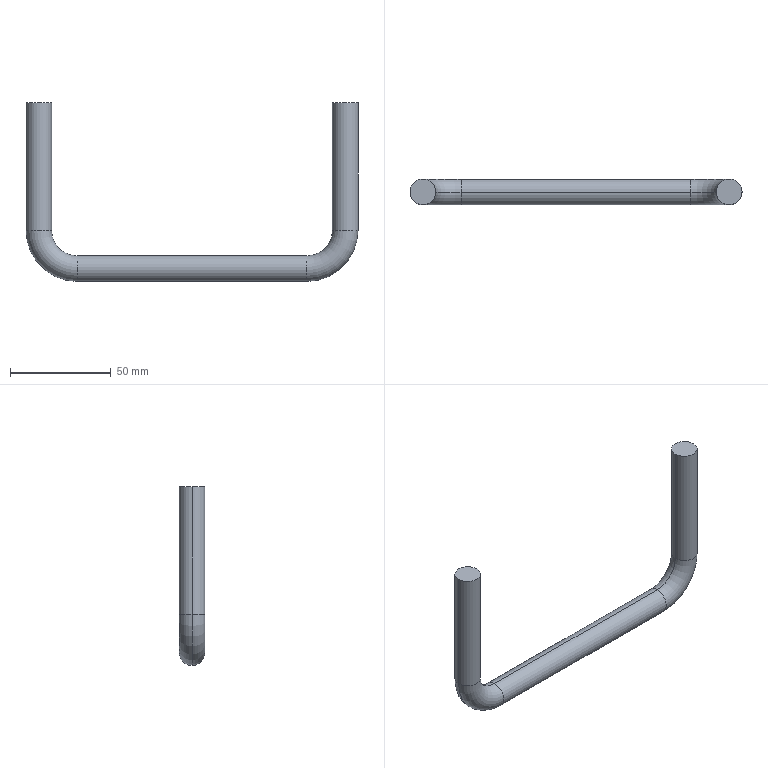Part | SolidWorks | features Sweep 1 | 1 solid | 12 faces | box 165.1 x 12.7 x 88.9 mm | volume 38148 mm3 | cylinder 6 | torus 4 | plane 2 | commonest cylinder face diameters 12.7 x6
STEP:
#1=CARTESIAN_POINT('',(-6.35,0.,-63.5));
#2=VERTEX_POINT('',#1);
#3=CARTESIAN_POINT('',(6.35,0.,-63.5));
#4=VERTEX_POINT('',#3);
#5=CARTESIAN_POINT('',(0.,0.,-63.5));
#6=DIRECTION('',(0.,0.,1.));
#7=DIRECTION('',(1.,0.,0.));
#8=AXIS2_PLACEMENT_3D('',#5,#6,#7);
#9=CIRCLE('',#8,6.35);
#10=EDGE_CURVE('',#2,#4,#9,.T.);
#11=ORIENTED_EDGE('',*,*,#10,.F.);
#12=CARTESIAN_POINT('',(19.05,0.,-88.9));
#13=VERTEX_POINT('',#12);
#14=CARTESIAN_POINT('',(19.05,0.,-63.5));
#15=DIRECTION('',(0.,-1.,0.));
#16=DIRECTION('',(0.,0.,-1.));
#17=AXIS2_PLACEMENT_3D('',#14,#15,#16);
#18=CIRCLE('',#17,25.4);
#19=EDGE_CURVE('',#2,#13,#18,.T.);
#20=ORIENTED_EDGE('',*,*,#19,.T.);
#21=CARTESIAN_POINT('',(19.05,0.,-76.2));
#22=VERTEX_POINT('',#21);
#23=CARTESIAN_POINT('',(19.05,0.,-82.55));
#24=DIRECTION('',(-1.,0.,0.));
#25=DIRECTION('',(0.,0.,1.));
#26=AXIS2_PLACEMENT_3D('',#23,#24,#25);
#27=CIRCLE('',#26,6.35);
#28=EDGE_CURVE('',#13,#22,#27,.T.);
#29=ORIENTED_EDGE('',*,*,#28,.T.);
#30=CARTESIAN_POINT('',(19.05,0.,-63.5));
#31=DIRECTION('',(0.,-1.,0.));
#32=DIRECTION('',(0.,0.,-1.));
#33=AXIS2_PLACEMENT_3D('',#30,#31,#32);
#34=CIRCLE('',#33,12.7);
#35=EDGE_CURVE('',#4,#22,#34,.T.);
#36=ORIENTED_EDGE('',*,*,#35,.F.);
#37=EDGE_LOOP('',(#11,#20,#29,#36));
#38=FACE_OUTER_BOUND('',#37,.T.);
#39=CARTESIAN_POINT('',(19.05,0.,-63.5));
#40=DIRECTION('',(0.,-1.,0.));
#41=DIRECTION('',(0.,0.,-1.));
#42=AXIS2_PLACEMENT_3D('',#39,#40,#41);
#43=TOROIDAL_SURFACE('',#42,19.05,6.35);
#44=ADVANCED_FACE('',(#38),#43,.T.);
#45=CARTESIAN_POINT('',(133.35,0.,-88.9));
#46=VERTEX_POINT('',#45);
#47=CARTESIAN_POINT('',(133.35,0.,-76.2));
#48=VERTEX_POINT('',#47);
#49=CARTESIAN_POINT('',(133.35,0.,-82.55));
#50=DIRECTION('',(-1.,0.,0.));
#51=DIRECTION('',(0.,0.,1.));
#52=AXIS2_PLACEMENT_3D('',#49,#50,#51);
#53=CIRCLE('',#52,6.35);
#54=EDGE_CURVE('',#46,#48,#53,.T.);
#55=ORIENTED_EDGE('',*,*,#54,.F.);
#56=CARTESIAN_POINT('',(158.75,0.,-63.5));
#57=VERTEX_POINT('',#56);
#58=CARTESIAN_POINT('',(133.35,0.,-63.5));
#59=DIRECTION('',(0.,-1.,0.));
#60=DIRECTION('',(0.,0.,-1.));
#61=AXIS2_PLACEMENT_3D('',#58,#59,#60);
#62=CIRCLE('',#61,25.4);
#63=EDGE_CURVE('',#46,#57,#62,.T.);
#64=ORIENTED_EDGE('',*,*,#63,.T.);
#65=CARTESIAN_POINT('',(146.05,0.,-63.5));
#66=VERTEX_POINT('',#65);
#67=CARTESIAN_POINT('',(152.4,0.,-63.5));
#68=DIRECTION('',(0.,0.,-1.));
#69=DIRECTION('',(-1.,0.,0.));
#70=AXIS2_PLACEMENT_3D('',#67,#68,#69);
#71=CIRCLE('',#70,6.35);
#72=EDGE_CURVE('',#57,#66,#71,.T.);
#73=ORIENTED_EDGE('',*,*,#72,.T.);
#74=CARTESIAN_POINT('',(133.35,0.,-63.5));
#75=DIRECTION('',(0.,-1.,0.));
#76=DIRECTION('',(0.,0.,-1.));
#77=AXIS2_PLACEMENT_3D('',#74,#75,#76);
#78=CIRCLE('',#77,12.7);
#79=EDGE_CURVE('',#48,#66,#78,.T.);
#80=ORIENTED_EDGE('',*,*,#79,.F.);
#81=EDGE_LOOP('',(#55,#64,#73,#80));
#82=FACE_OUTER_BOUND('',#81,.T.);
#83=CARTESIAN_POINT('',(133.35,0.,-63.5));
#84=DIRECTION('',(0.,-1.,0.));
#85=DIRECTION('',(0.,0.,-1.));
#86=AXIS2_PLACEMENT_3D('',#83,#84,#85);
#87=TOROIDAL_SURFACE('',#86,19.05,6.35);
#88=ADVANCED_FACE('',(#82),#87,.T.);
#89=CARTESIAN_POINT('',(0.,0.,-63.5));
#90=DIRECTION('',(0.,0.,1.));
#91=DIRECTION('',(1.,0.,0.));
#92=AXIS2_PLACEMENT_3D('',#89,#90,#91);
#93=CIRCLE('',#92,6.35);
#94=EDGE_CURVE('',#4,#2,#93,.T.);
#95=ORIENTED_EDGE('',*,*,#94,.T.);
#96=CARTESIAN_POINT('',(-6.35,0.,0.));
#97=VERTEX_POINT('',#96);
#98=CARTESIAN_POINT('',(-6.35,0.,-63.5));
#99=DIRECTION('',(0.,0.,1.));
#100=VECTOR('',#99,1000.);
#101=LINE('',#98,#100);
#102=EDGE_CURVE('',#2,#97,#101,.T.);
#103=ORIENTED_EDGE('',*,*,#102,.T.);
#104=CARTESIAN_POINT('',(6.35,0.,0.));
#105=VERTEX_POINT('',#104);
#106=CARTESIAN_POINT('',(0.,0.,0.));
#107=DIRECTION('',(0.,0.,1.));
#108=DIRECTION('',(1.,0.,0.));
#109=AXIS2_PLACEMENT_3D('',#106,#107,#108);
#110=CIRCLE('',#109,6.35);
#111=EDGE_CURVE('',#105,#97,#110,.T.);
#112=ORIENTED_EDGE('',*,*,#111,.F.);
#113=CARTESIAN_POINT('',(6.35,0.,-63.5));
#114=DIRECTION('',(0.,0.,1.));
#115=VECTOR('',#114,1000.);
#116=LINE('',#113,#115);
#117=EDGE_CURVE('',#4,#105,#116,.T.);
#118=ORIENTED_EDGE('',*,*,#117,.F.);
#119=EDGE_LOOP('',(#95,#103,#112,#118));
#120=FACE_OUTER_BOUND('',#119,.T.);
#121=CARTESIAN_POINT('',(0.,0.,-63.5));
#122=DIRECTION('',(0.,0.,1.));
#123=DIRECTION('',(1.,0.,0.));
#124=AXIS2_PLACEMENT_3D('',#121,#122,#123);
#125=CYLINDRICAL_SURFACE('',#124,6.35);
#126=ADVANCED_FACE('',(#120),#125,.T.);
#127=CARTESIAN_POINT('',(19.05,0.,-82.55));
#128=DIRECTION('',(-1.,0.,0.));
#129=DIRECTION('',(0.,0.,1.));
#130=AXIS2_PLACEMENT_3D('',#127,#128,#129);
#131=CIRCLE('',#130,6.35);
#132=EDGE_CURVE('',#22,#13,#131,.T.);
#133=ORIENTED_EDGE('',*,*,#132,.F.);
#134=CARTESIAN_POINT('',(19.05,0.,-76.2));
#135=DIRECTION('',(1.,0.,0.));
#136=VECTOR('',#135,1000.);
#137=LINE('',#134,#136);
#138=EDGE_CURVE('',#22,#48,#137,.T.);
#139=ORIENTED_EDGE('',*,*,#138,.T.);
#140=CARTESIAN_POINT('',(133.35,0.,-82.55));
#141=DIRECTION('',(-1.,0.,0.));
#142=DIRECTION('',(0.,0.,1.));
#143=AXIS2_PLACEMENT_3D('',#140,#141,#142);
#144=CIRCLE('',#143,6.35);
#145=EDGE_CURVE('',#48,#46,#144,.T.);
#146=ORIENTED_EDGE('',*,*,#145,.T.);
#147=CARTESIAN_POINT('',(19.05,0.,-88.9));
#148=DIRECTION('',(1.,0.,0.));
#149=VECTOR('',#148,1000.);
#150=LINE('',#147,#149);
#151=EDGE_CURVE('',#13,#46,#150,.T.);
#152=ORIENTED_EDGE('',*,*,#151,.F.);
#153=EDGE_LOOP('',(#133,#139,#146,#152));
#154=FACE_OUTER_BOUND('',#153,.T.);
#155=CARTESIAN_POINT('',(19.05,0.,-82.55));
#156=DIRECTION('',(1.,0.,0.));
#157=DIRECTION('',(0.,0.,-1.));
#158=AXIS2_PLACEMENT_3D('',#155,#156,#157);
#159=CYLINDRICAL_SURFACE('',#158,6.35);
#160=ADVANCED_FACE('',(#154),#159,.T.);
#161=CARTESIAN_POINT('',(152.4,0.,-63.5));
#162=DIRECTION('',(0.,0.,-1.));
#163=DIRECTION('',(-1.,0.,0.));
#164=AXIS2_PLACEMENT_3D('',#161,#162,#163);
#165=CIRCLE('',#164,6.35);
#166=EDGE_CURVE('',#66,#57,#165,.T.);
#167=ORIENTED_EDGE('',*,*,#166,.F.);
#168=CARTESIAN_POINT('',(146.05,0.,0.));
#169=VERTEX_POINT('',#168);
#170=CARTESIAN_POINT('',(146.05,0.,-63.5));
#171=DIRECTION('',(0.,0.,1.));
#172=VECTOR('',#171,1000.);
#173=LINE('',#170,#172);
#174=EDGE_CURVE('',#66,#169,#173,.T.);
#175=ORIENTED_EDGE('',*,*,#174,.T.);
#176=CARTESIAN_POINT('',(158.75,0.,0.));
#177=VERTEX_POINT('',#176);
#178=CARTESIAN_POINT('',(152.4,0.,0.));
#179=DIRECTION('',(0.,0.,-1.));
#180=DIRECTION('',(-1.,0.,0.));
#181=AXIS2_PLACEMENT_3D('',#178,#179,#180);
#182=CIRCLE('',#181,6.35);
#183=EDGE_CURVE('',#169,#177,#182,.T.);
#184=ORIENTED_EDGE('',*,*,#183,.T.);
#185=CARTESIAN_POINT('',(158.75,0.,-63.5));
#186=DIRECTION('',(0.,0.,1.));
#187=VECTOR('',#186,1000.);
#188=LINE('',#185,#187);
#189=EDGE_CURVE('',#57,#177,#188,.T.);
#190=ORIENTED_EDGE('',*,*,#189,.F.);
#191=EDGE_LOOP('',(#167,#175,#184,#190));
#192=FACE_OUTER_BOUND('',#191,.T.);
#193=CARTESIAN_POINT('',(152.4,0.,-63.5));
#194=DIRECTION('',(0.,0.,1.));
#195=DIRECTION('',(1.,0.,0.));
#196=AXIS2_PLACEMENT_3D('',#193,#194,#195);
#197=CYLINDRICAL_SURFACE('',#196,6.35);
#198=ADVANCED_FACE('',(#192),#197,.T.);
#199=ORIENTED_EDGE('',*,*,#174,.F.);
#200=ORIENTED_EDGE('',*,*,#72,.F.);
#201=ORIENTED_EDGE('',*,*,#189,.T.);
#202=CARTESIAN_POINT('',(152.4,0.,0.));
#203=DIRECTION('',(0.,0.,-1.));
#204=DIRECTION('',(-1.,0.,0.));
#205=AXIS2_PLACEMENT_3D('',#202,#203,#204);
#206=CIRCLE('',#205,6.35);
#207=EDGE_CURVE('',#177,#169,#206,.T.);
#208=ORIENTED_EDGE('',*,*,#207,.T.);
#209=EDGE_LOOP('',(#199,#200,#201,#208));
#210=FACE_OUTER_BOUND('',#209,.T.);
#211=CARTESIAN_POINT('',(152.4,0.,-63.5));
#212=DIRECTION('',(0.,0.,1.));
#213=DIRECTION('',(1.,0.,0.));
#214=AXIS2_PLACEMENT_3D('',#211,#212,#213);
#215=CYLINDRICAL_SURFACE('',#214,6.35);
#216=ADVANCED_FACE('',(#210),#215,.T.);
#217=ORIENTED_EDGE('',*,*,#63,.F.);
#218=ORIENTED_EDGE('',*,*,#145,.F.);
#219=ORIENTED_EDGE('',*,*,#79,.T.);
#220=ORIENTED_EDGE('',*,*,#166,.T.);
#221=EDGE_LOOP('',(#217,#218,#219,#220));
#222=FACE_OUTER_BOUND('',#221,.T.);
#223=CARTESIAN_POINT('',(133.35,0.,-63.5));
#224=DIRECTION('',(0.,-1.,0.));
#225=DIRECTION('',(0.,0.,-1.));
#226=AXIS2_PLACEMENT_3D('',#223,#224,#225);
#227=TOROIDAL_SURFACE('',#226,19.05,6.35);
#228=ADVANCED_FACE('',(#222),#227,.T.);
#229=ORIENTED_EDGE('',*,*,#138,.F.);
#230=ORIENTED_EDGE('',*,*,#28,.F.);
#231=ORIENTED_EDGE('',*,*,#151,.T.);
#232=ORIENTED_EDGE('',*,*,#54,.T.);
#233=EDGE_LOOP('',(#229,#230,#231,#232));
#234=FACE_OUTER_BOUND('',#233,.T.);
#235=CARTESIAN_POINT('',(19.05,0.,-82.55));
#236=DIRECTION('',(1.,0.,0.));
#237=DIRECTION('',(0.,0.,-1.));
#238=AXIS2_PLACEMENT_3D('',#235,#236,#237);
#239=CYLINDRICAL_SURFACE('',#238,6.35);
#240=ADVANCED_FACE('',(#234),#239,.T.);
#241=ORIENTED_EDGE('',*,*,#19,.F.);
#242=ORIENTED_EDGE('',*,*,#94,.F.);
#243=ORIENTED_EDGE('',*,*,#35,.T.);
#244=ORIENTED_EDGE('',*,*,#132,.T.);
#245=EDGE_LOOP('',(#241,#242,#243,#244));
#246=FACE_OUTER_BOUND('',#245,.T.);
#247=CARTESIAN_POINT('',(19.05,0.,-63.5));
#248=DIRECTION('',(0.,-1.,0.));
#249=DIRECTION('',(0.,0.,-1.));
#250=AXIS2_PLACEMENT_3D('',#247,#248,#249);
#251=TOROIDAL_SURFACE('',#250,19.05,6.35);
#252=ADVANCED_FACE('',(#246),#251,.T.);
#253=ORIENTED_EDGE('',*,*,#102,.F.);
#254=ORIENTED_EDGE('',*,*,#10,.T.);
#255=ORIENTED_EDGE('',*,*,#117,.T.);
#256=CARTESIAN_POINT('',(0.,0.,0.));
#257=DIRECTION('',(0.,0.,1.));
#258=DIRECTION('',(1.,0.,0.));
#259=AXIS2_PLACEMENT_3D('',#256,#257,#258);
#260=CIRCLE('',#259,6.35);
#261=EDGE_CURVE('',#97,#105,#260,.T.);
#262=ORIENTED_EDGE('',*,*,#261,.F.);
#263=EDGE_LOOP('',(#253,#254,#255,#262));
#264=FACE_OUTER_BOUND('',#263,.T.);
#265=CARTESIAN_POINT('',(0.,0.,-63.5));
#266=DIRECTION('',(0.,0.,1.));
#267=DIRECTION('',(1.,0.,0.));
#268=AXIS2_PLACEMENT_3D('',#265,#266,#267);
#269=CYLINDRICAL_SURFACE('',#268,6.35);
#270=ADVANCED_FACE('',(#264),#269,.T.);
#271=ORIENTED_EDGE('',*,*,#207,.F.);
#272=ORIENTED_EDGE('',*,*,#183,.F.);
#273=EDGE_LOOP('',(#271,#272));
#274=FACE_OUTER_BOUND('',#273,.T.);
#275=CARTESIAN_POINT('',(152.4,0.,0.));
#276=DIRECTION('',(0.,0.,-1.));
#277=DIRECTION('',(-1.,0.,0.));
#278=AXIS2_PLACEMENT_3D('',#275,#276,#277);
#279=PLANE('',#278);
#280=ADVANCED_FACE('',(#274),#279,.F.);
#281=ORIENTED_EDGE('',*,*,#111,.T.);
#282=ORIENTED_EDGE('',*,*,#261,.T.);
#283=EDGE_LOOP('',(#281,#282));
#284=FACE_OUTER_BOUND('',#283,.T.);
#285=CARTESIAN_POINT('',(0.,0.,0.));
#286=DIRECTION('',(0.,0.,1.));
#287=DIRECTION('',(1.,0.,0.));
#288=AXIS2_PLACEMENT_3D('',#285,#286,#287);
#289=PLANE('',#288);
#290=ADVANCED_FACE('',(#284),#289,.T.);
#291=CLOSED_SHELL('',(#44,#88,#126,#160,#198,#216,#228,#240,#252,#270,#280,#290));
#292=MANIFOLD_SOLID_BREP('',#291);
#293=CARTESIAN_POINT('',(0.,0.,0.));
#294=DIRECTION('',(0.,0.,1.));
#295=DIRECTION('',(1.,0.,0.));
#296=AXIS2_PLACEMENT_3D('',#293,#294,#295);
#297=(LENGTH_UNIT()NAMED_UNIT(*)SI_UNIT(.MILLI.,.METRE.));
#298=UNCERTAINTY_MEASURE_WITH_UNIT(LENGTH_MEASURE(0.00001),#297,'','');
#299=(NAMED_UNIT(*)PLANE_ANGLE_UNIT()SI_UNIT($,.RADIAN.));
#300=(NAMED_UNIT(*)SI_UNIT($,.STERADIAN.)SOLID_ANGLE_UNIT());
#301=(GEOMETRIC_REPRESENTATION_CONTEXT(3)GLOBAL_UNCERTAINTY_ASSIGNED_CONTEXT((#298))GLOBAL_UNIT_ASSIGNED_CONTEXT((#297,#299,#300))REPRESENTATION_CONTEXT('',''));
#302=ADVANCED_BREP_SHAPE_REPRESENTATION('',(#292,#296),#301);